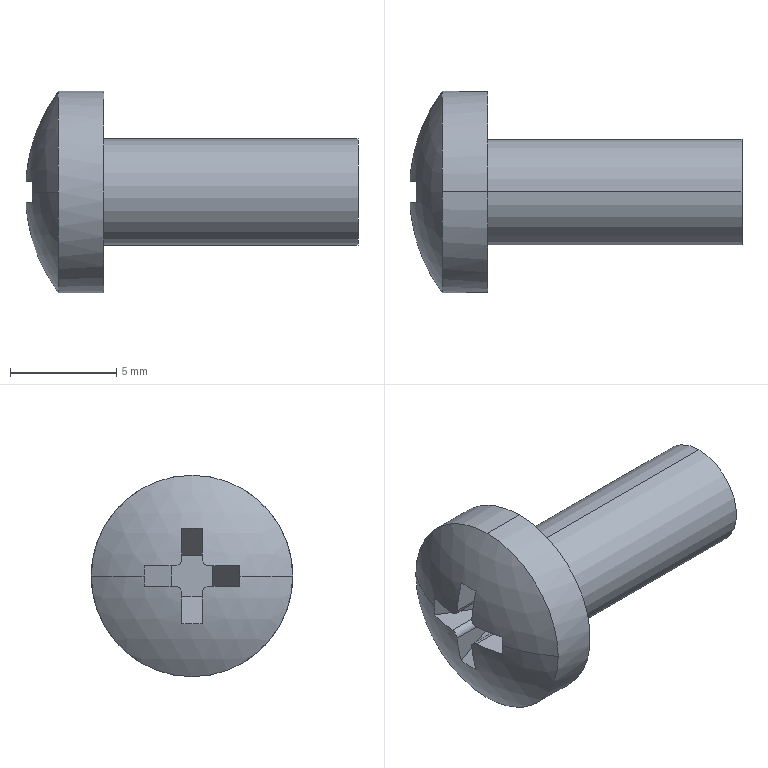Part | SolidWorks | features BaseBody 1 | 1 solid | 25 faces | box 15.658 x 9.5 x 9.5 mm | volume 430.614 mm3 | plane 15 | cylinder 8 | sphere 2 | commonest cylinder face diameters 0.6 x4 5 x2 9.5 x2
STEP:
#1=CARTESIAN_POINT('',(1.563,4.75,0.));
#2=VERTEX_POINT('',#1);
#3=CARTESIAN_POINT('',(1.563,0.,4.75));
#4=VERTEX_POINT('',#3);
#5=CARTESIAN_POINT('',(1.563,0.,0.));
#6=DIRECTION('',(1.,0.,0.));
#7=DIRECTION('',(0.,0.,-1.));
#8=AXIS2_PLACEMENT_3D('',#5,#6,#7);
#9=CIRCLE('',#8,4.75);
#10=EDGE_CURVE('',#2,#4,#9,.T.);
#11=ORIENTED_EDGE('',*,*,#10,.T.);
#12=CARTESIAN_POINT('',(3.7,0.,4.75));
#13=VERTEX_POINT('',#12);
#14=CARTESIAN_POINT('',(4.516,0.,4.75));
#15=DIRECTION('',(1.,0.,0.));
#16=VECTOR('',#15,1000.);
#17=LINE('',#14,#16);
#18=EDGE_CURVE('',#4,#13,#17,.T.);
#19=ORIENTED_EDGE('',*,*,#18,.T.);
#20=CARTESIAN_POINT('',(3.7,0.,-4.75));
#21=VERTEX_POINT('',#20);
#22=CARTESIAN_POINT('',(3.7,0.,0.));
#23=DIRECTION('',(1.,0.,0.));
#24=DIRECTION('',(0.,0.,-1.));
#25=AXIS2_PLACEMENT_3D('',#22,#23,#24);
#26=CIRCLE('',#25,4.75);
#27=EDGE_CURVE('',#21,#13,#26,.T.);
#28=ORIENTED_EDGE('',*,*,#27,.F.);
#29=CARTESIAN_POINT('',(1.563,0.,-4.75));
#30=VERTEX_POINT('',#29);
#31=CARTESIAN_POINT('',(4.516,0.,-4.75));
#32=DIRECTION('',(1.,0.,0.));
#33=VECTOR('',#32,1000.);
#34=LINE('',#31,#33);
#35=EDGE_CURVE('',#30,#21,#34,.T.);
#36=ORIENTED_EDGE('',*,*,#35,.F.);
#37=CARTESIAN_POINT('',(1.563,0.,0.));
#38=DIRECTION('',(1.,0.,0.));
#39=DIRECTION('',(0.,0.,-1.));
#40=AXIS2_PLACEMENT_3D('',#37,#38,#39);
#41=CIRCLE('',#40,4.75);
#42=EDGE_CURVE('',#30,#2,#41,.T.);
#43=ORIENTED_EDGE('',*,*,#42,.T.);
#44=EDGE_LOOP('',(#11,#19,#28,#36,#43));
#45=FACE_OUTER_BOUND('',#44,.T.);
#46=CARTESIAN_POINT('',(4.516,0.,0.));
#47=DIRECTION('',(1.,0.,0.));
#48=DIRECTION('',(0.,0.,-1.));
#49=AXIS2_PLACEMENT_3D('',#46,#47,#48);
#50=CYLINDRICAL_SURFACE('',#49,4.75);
#51=ADVANCED_FACE('',(#45),#50,.T.);
#52=CARTESIAN_POINT('',(3.7,0.,-2.5));
#53=VERTEX_POINT('',#52);
#54=CARTESIAN_POINT('',(3.7,0.,2.5));
#55=VERTEX_POINT('',#54);
#56=CARTESIAN_POINT('',(3.7,0.,0.));
#57=DIRECTION('',(1.,0.,0.));
#58=DIRECTION('',(0.,0.,-1.));
#59=AXIS2_PLACEMENT_3D('',#56,#57,#58);
#60=CIRCLE('',#59,2.5);
#61=EDGE_CURVE('',#53,#55,#60,.T.);
#62=ORIENTED_EDGE('',*,*,#61,.T.);
#63=CARTESIAN_POINT('',(15.7,0.,2.5));
#64=VERTEX_POINT('',#63);
#65=CARTESIAN_POINT('',(4.516,0.,2.5));
#66=DIRECTION('',(1.,0.,0.));
#67=VECTOR('',#66,1000.);
#68=LINE('',#65,#67);
#69=EDGE_CURVE('',#55,#64,#68,.T.);
#70=ORIENTED_EDGE('',*,*,#69,.T.);
#71=CARTESIAN_POINT('',(15.7,0.,-2.5));
#72=VERTEX_POINT('',#71);
#73=CARTESIAN_POINT('',(15.7,0.,0.));
#74=DIRECTION('',(1.,0.,0.));
#75=DIRECTION('',(0.,0.,-1.));
#76=AXIS2_PLACEMENT_3D('',#73,#74,#75);
#77=CIRCLE('',#76,2.5);
#78=EDGE_CURVE('',#72,#64,#77,.T.);
#79=ORIENTED_EDGE('',*,*,#78,.F.);
#80=CARTESIAN_POINT('',(4.516,0.,-2.5));
#81=DIRECTION('',(1.,0.,0.));
#82=VECTOR('',#81,1000.);
#83=LINE('',#80,#82);
#84=EDGE_CURVE('',#53,#72,#83,.T.);
#85=ORIENTED_EDGE('',*,*,#84,.F.);
#86=EDGE_LOOP('',(#62,#70,#79,#85));
#87=FACE_OUTER_BOUND('',#86,.T.);
#88=CARTESIAN_POINT('',(4.516,0.,0.));
#89=DIRECTION('',(1.,0.,0.));
#90=DIRECTION('',(0.,0.,-1.));
#91=AXIS2_PLACEMENT_3D('',#88,#89,#90);
#92=CYLINDRICAL_SURFACE('',#91,2.5);
#93=ADVANCED_FACE('',(#87),#92,.T.);
#94=CARTESIAN_POINT('',(1.563,-4.75,0.));
#95=VERTEX_POINT('',#94);
#96=CARTESIAN_POINT('',(1.563,0.,0.));
#97=DIRECTION('',(1.,0.,0.));
#98=DIRECTION('',(0.,0.,-1.));
#99=AXIS2_PLACEMENT_3D('',#96,#97,#98);
#100=CIRCLE('',#99,4.75);
#101=EDGE_CURVE('',#95,#30,#100,.T.);
#102=ORIENTED_EDGE('',*,*,#101,.F.);
#103=CARTESIAN_POINT('',(0.3263,-2.262,0.));
#104=VERTEX_POINT('',#103);
#105=CARTESIAN_POINT('',(8.,0.,0.));
#106=DIRECTION('',(0.,0.,-1.));
#107=DIRECTION('',(0.,1.,0.));
#108=AXIS2_PLACEMENT_3D('',#105,#106,#107);
#109=CIRCLE('',#108,8.);
#110=EDGE_CURVE('',#95,#104,#109,.T.);
#111=ORIENTED_EDGE('',*,*,#110,.T.);
#112=CARTESIAN_POINT('',(0.3397,-2.254,-0.49));
#113=VERTEX_POINT('',#112);
#114=CARTESIAN_POINT('',(7.061,1.627,0.));
#115=DIRECTION('',(0.5,-0.866,0.));
#116=DIRECTION('',(-0.866,-0.5,0.));
#117=AXIS2_PLACEMENT_3D('',#114,#115,#116);
#118=CIRCLE('',#117,7.776);
#119=EDGE_CURVE('',#104,#113,#118,.T.);
#120=ORIENTED_EDGE('',*,*,#119,.T.);
#121=CARTESIAN_POINT('',(0.0542,-0.79,-0.49));
#122=VERTEX_POINT('',#121);
#123=CARTESIAN_POINT('',(8.,0.,-0.49));
#124=DIRECTION('',(0.,0.,-1.));
#125=DIRECTION('',(1.,0.,0.));
#126=AXIS2_PLACEMENT_3D('',#123,#124,#125);
#127=CIRCLE('',#126,7.985);
#128=EDGE_CURVE('',#113,#122,#127,.T.);
#129=ORIENTED_EDGE('',*,*,#128,.T.);
#130=CARTESIAN_POINT('',(0.0542,-0.49,-0.79));
#131=VERTEX_POINT('',#130);
#132=CARTESIAN_POINT('',(0.0542,-0.79,-0.49));
#133=CARTESIAN_POINT('',(0.04634,-0.711,-0.49));
#134=CARTESIAN_POINT('',(0.04186,-0.6334,-0.5224));
#135=CARTESIAN_POINT('',(0.04185,-0.5225,-0.6332));
#136=CARTESIAN_POINT('',(0.04634,-0.49,-0.711));
#137=CARTESIAN_POINT('',(0.0542,-0.49,-0.79));
#138=B_SPLINE_CURVE_WITH_KNOTS('',3,(#132,#133,#134,#135,#136,#137),.UNSPECIFIED.,.F.,.F.,(4,2,4),(0.,0.0002348,0.0004695),.UNSPECIFIED.);
#139=EDGE_CURVE('',#122,#131,#138,.T.);
#140=ORIENTED_EDGE('',*,*,#139,.T.);
#141=CARTESIAN_POINT('',(0.3397,-0.49,-2.254));
#142=VERTEX_POINT('',#141);
#143=CARTESIAN_POINT('',(8.,-0.49,0.));
#144=DIRECTION('',(0.,-1.,0.));
#145=DIRECTION('',(0.,0.,1.));
#146=AXIS2_PLACEMENT_3D('',#143,#144,#145);
#147=CIRCLE('',#146,7.985);
#148=EDGE_CURVE('',#131,#142,#147,.T.);
#149=ORIENTED_EDGE('',*,*,#148,.T.);
#150=CARTESIAN_POINT('',(0.3397,0.49,-2.254));
#151=VERTEX_POINT('',#150);
#152=CARTESIAN_POINT('',(7.061,0.,1.627));
#153=DIRECTION('',(0.5,0.,-0.866));
#154=DIRECTION('',(0.866,0.,0.5));
#155=AXIS2_PLACEMENT_3D('',#152,#153,#154);
#156=CIRCLE('',#155,7.776);
#157=EDGE_CURVE('',#142,#151,#156,.T.);
#158=ORIENTED_EDGE('',*,*,#157,.T.);
#159=CARTESIAN_POINT('',(0.0542,0.49,-0.79));
#160=VERTEX_POINT('',#159);
#161=CARTESIAN_POINT('',(8.,0.49,0.));
#162=DIRECTION('',(0.,1.,0.));
#163=DIRECTION('',(0.,0.,-1.));
#164=AXIS2_PLACEMENT_3D('',#161,#162,#163);
#165=CIRCLE('',#164,7.985);
#166=EDGE_CURVE('',#151,#160,#165,.T.);
#167=ORIENTED_EDGE('',*,*,#166,.T.);
#168=CARTESIAN_POINT('',(0.0542,0.79,-0.49));
#169=VERTEX_POINT('',#168);
#170=CARTESIAN_POINT('',(0.0542,0.49,-0.79));
#171=CARTESIAN_POINT('',(0.04634,0.49,-0.711));
#172=CARTESIAN_POINT('',(0.04186,0.5224,-0.6334));
#173=CARTESIAN_POINT('',(0.04185,0.6332,-0.5225));
#174=CARTESIAN_POINT('',(0.04634,0.711,-0.49));
#175=CARTESIAN_POINT('',(0.0542,0.79,-0.49));
#176=B_SPLINE_CURVE_WITH_KNOTS('',3,(#170,#171,#172,#173,#174,#175),.UNSPECIFIED.,.F.,.F.,(4,2,4),(0.,0.0002348,0.0004695),.UNSPECIFIED.);
#177=EDGE_CURVE('',#160,#169,#176,.T.);
#178=ORIENTED_EDGE('',*,*,#177,.T.);
#179=CARTESIAN_POINT('',(0.3397,2.254,-0.49));
#180=VERTEX_POINT('',#179);
#181=CARTESIAN_POINT('',(8.,0.,-0.49));
#182=DIRECTION('',(0.,0.,-1.));
#183=DIRECTION('',(1.,0.,0.));
#184=AXIS2_PLACEMENT_3D('',#181,#182,#183);
#185=CIRCLE('',#184,7.985);
#186=EDGE_CURVE('',#169,#180,#185,.T.);
#187=ORIENTED_EDGE('',*,*,#186,.T.);
#188=CARTESIAN_POINT('',(0.3263,2.262,0.));
#189=VERTEX_POINT('',#188);
#190=CARTESIAN_POINT('',(7.061,-1.627,0.));
#191=DIRECTION('',(0.5,0.866,0.));
#192=DIRECTION('',(0.866,-0.5,0.));
#193=AXIS2_PLACEMENT_3D('',#190,#191,#192);
#194=CIRCLE('',#193,7.776);
#195=EDGE_CURVE('',#180,#189,#194,.T.);
#196=ORIENTED_EDGE('',*,*,#195,.T.);
#197=CARTESIAN_POINT('',(8.,0.,0.));
#198=DIRECTION('',(0.,0.,1.));
#199=DIRECTION('',(1.,0.,0.));
#200=AXIS2_PLACEMENT_3D('',#197,#198,#199);
#201=CIRCLE('',#200,8.);
#202=EDGE_CURVE('',#2,#189,#201,.T.);
#203=ORIENTED_EDGE('',*,*,#202,.F.);
#204=ORIENTED_EDGE('',*,*,#42,.F.);
#205=EDGE_LOOP('',(#102,#111,#120,#129,#140,#149,#158,#167,#178,#187,#196,#203,#204));
#206=FACE_OUTER_BOUND('',#205,.T.);
#207=CARTESIAN_POINT('',(8.,0.,0.));
#208=DIRECTION('',(0.,0.,-1.));
#209=DIRECTION('',(0.,1.,0.));
#210=AXIS2_PLACEMENT_3D('',#207,#208,#209);
#211=SPHERICAL_SURFACE('',#210,8.);
#212=ADVANCED_FACE('',(#206),#211,.T.);
#213=CARTESIAN_POINT('',(2.59,0.79,-0.49));
#214=VERTEX_POINT('',#213);
#215=CARTESIAN_POINT('',(2.59,0.49,-0.79));
#216=VERTEX_POINT('',#215);
#217=CARTESIAN_POINT('',(2.59,0.79,-0.79));
#218=DIRECTION('',(1.,0.,0.));
#219=DIRECTION('',(0.,0.,-1.));
#220=AXIS2_PLACEMENT_3D('',#217,#218,#219);
#221=CIRCLE('',#220,0.3);
#222=EDGE_CURVE('',#214,#216,#221,.T.);
#223=ORIENTED_EDGE('',*,*,#222,.F.);
#224=CARTESIAN_POINT('',(2.59,0.79,-0.49));
#225=DIRECTION('',(1.,0.,0.));
#226=VECTOR('',#225,1000.);
#227=LINE('',#224,#226);
#228=EDGE_CURVE('',#169,#214,#227,.T.);
#229=ORIENTED_EDGE('',*,*,#228,.F.);
#230=ORIENTED_EDGE('',*,*,#177,.F.);
#231=CARTESIAN_POINT('',(2.59,0.49,-0.79));
#232=DIRECTION('',(-1.,0.,0.));
#233=VECTOR('',#232,1000.);
#234=LINE('',#231,#233);
#235=EDGE_CURVE('',#216,#160,#234,.T.);
#236=ORIENTED_EDGE('',*,*,#235,.F.);
#237=EDGE_LOOP('',(#223,#229,#230,#236));
#238=FACE_OUTER_BOUND('',#237,.T.);
#239=CARTESIAN_POINT('',(2.59,0.79,-0.79));
#240=DIRECTION('',(-1.,0.,0.));
#241=DIRECTION('',(0.,0.,1.));
#242=AXIS2_PLACEMENT_3D('',#239,#240,#241);
#243=CYLINDRICAL_SURFACE('',#242,0.3);
#244=ADVANCED_FACE('',(#238),#243,.T.);
#245=CARTESIAN_POINT('',(2.59,0.49,0.79));
#246=VERTEX_POINT('',#245);
#247=CARTESIAN_POINT('',(2.59,0.79,0.49));
#248=VERTEX_POINT('',#247);
#249=CARTESIAN_POINT('',(2.59,0.79,0.79));
#250=DIRECTION('',(1.,0.,0.));
#251=DIRECTION('',(0.,0.,-1.));
#252=AXIS2_PLACEMENT_3D('',#249,#250,#251);
#253=CIRCLE('',#252,0.3);
#254=EDGE_CURVE('',#246,#248,#253,.T.);
#255=ORIENTED_EDGE('',*,*,#254,.F.);
#256=CARTESIAN_POINT('',(0.0542,0.49,0.79));
#257=VERTEX_POINT('',#256);
#258=CARTESIAN_POINT('',(2.59,0.49,0.79));
#259=DIRECTION('',(1.,0.,0.));
#260=VECTOR('',#259,1000.);
#261=LINE('',#258,#260);
#262=EDGE_CURVE('',#257,#246,#261,.T.);
#263=ORIENTED_EDGE('',*,*,#262,.F.);
#264=CARTESIAN_POINT('',(0.0542,0.79,0.49));
#265=VERTEX_POINT('',#264);
#266=CARTESIAN_POINT('',(0.0542,0.79,0.49));
#267=CARTESIAN_POINT('',(0.04634,0.711,0.49));
#268=CARTESIAN_POINT('',(0.04186,0.6334,0.5224));
#269=CARTESIAN_POINT('',(0.04185,0.5225,0.6332));
#270=CARTESIAN_POINT('',(0.04634,0.49,0.711));
#271=CARTESIAN_POINT('',(0.0542,0.49,0.79));
#272=B_SPLINE_CURVE_WITH_KNOTS('',3,(#266,#267,#268,#269,#270,#271),.UNSPECIFIED.,.F.,.F.,(4,2,4),(0.,0.0002348,0.0004695),.UNSPECIFIED.);
#273=EDGE_CURVE('',#265,#257,#272,.T.);
#274=ORIENTED_EDGE('',*,*,#273,.F.);
#275=CARTESIAN_POINT('',(2.59,0.79,0.49));
#276=DIRECTION('',(-1.,0.,0.));
#277=VECTOR('',#276,1000.);
#278=LINE('',#275,#277);
#279=EDGE_CURVE('',#248,#265,#278,.T.);
#280=ORIENTED_EDGE('',*,*,#279,.F.);
#281=EDGE_LOOP('',(#255,#263,#274,#280));
#282=FACE_OUTER_BOUND('',#281,.T.);
#283=CARTESIAN_POINT('',(2.59,0.79,0.79));
#284=DIRECTION('',(-1.,0.,0.));
#285=DIRECTION('',(0.,0.,1.));
#286=AXIS2_PLACEMENT_3D('',#283,#284,#285);
#287=CYLINDRICAL_SURFACE('',#286,0.3);
#288=ADVANCED_FACE('',(#282),#287,.T.);
#289=CARTESIAN_POINT('',(2.59,-0.49,-0.79));
#290=VERTEX_POINT('',#289);
#291=CARTESIAN_POINT('',(2.59,-0.79,-0.49));
#292=VERTEX_POINT('',#291);
#293=CARTESIAN_POINT('',(2.59,-0.79,-0.79));
#294=DIRECTION('',(1.,0.,0.));
#295=DIRECTION('',(0.,0.,-1.));
#296=AXIS2_PLACEMENT_3D('',#293,#294,#295);
#297=CIRCLE('',#296,0.3);
#298=EDGE_CURVE('',#290,#292,#297,.T.);
#299=ORIENTED_EDGE('',*,*,#298,.F.);
#300=CARTESIAN_POINT('',(2.59,-0.49,-0.79));
#301=DIRECTION('',(1.,0.,0.));
#302=VECTOR('',#301,1000.);
#303=LINE('',#300,#302);
#304=EDGE_CURVE('',#131,#290,#303,.T.);
#305=ORIENTED_EDGE('',*,*,#304,.F.);
#306=ORIENTED_EDGE('',*,*,#139,.F.);
#307=CARTESIAN_POINT('',(2.59,-0.79,-0.49));
#308=DIRECTION('',(-1.,0.,0.));
#309=VECTOR('',#308,1000.);
#310=LINE('',#307,#309);
#311=EDGE_CURVE('',#292,#122,#310,.T.);
#312=ORIENTED_EDGE('',*,*,#311,.F.);
#313=EDGE_LOOP('',(#299,#305,#306,#312));
#314=FACE_OUTER_BOUND('',#313,.T.);
#315=CARTESIAN_POINT('',(2.59,-0.79,-0.79));
#316=DIRECTION('',(-1.,0.,0.));
#317=DIRECTION('',(0.,0.,1.));
#318=AXIS2_PLACEMENT_3D('',#315,#316,#317);
#319=CYLINDRICAL_SURFACE('',#318,0.3);
#320=ADVANCED_FACE('',(#314),#319,.T.);
#321=CARTESIAN_POINT('',(2.59,-0.79,0.49));
#322=VERTEX_POINT('',#321);
#323=CARTESIAN_POINT('',(2.59,-0.49,0.79));
#324=VERTEX_POINT('',#323);
#325=CARTESIAN_POINT('',(2.59,-0.79,0.79));
#326=DIRECTION('',(1.,0.,0.));
#327=DIRECTION('',(0.,0.,-1.));
#328=AXIS2_PLACEMENT_3D('',#325,#326,#327);
#329=CIRCLE('',#328,0.3);
#330=EDGE_CURVE('',#322,#324,#329,.T.);
#331=ORIENTED_EDGE('',*,*,#330,.F.);
#332=CARTESIAN_POINT('',(0.0542,-0.79,0.49));
#333=VERTEX_POINT('',#332);
#334=CARTESIAN_POINT('',(2.59,-0.79,0.49));
#335=DIRECTION('',(1.,0.,0.));
#336=VECTOR('',#335,1000.);
#337=LINE('',#334,#336);
#338=EDGE_CURVE('',#333,#322,#337,.T.);
#339=ORIENTED_EDGE('',*,*,#338,.F.);
#340=CARTESIAN_POINT('',(0.0542,-0.49,0.79));
#341=VERTEX_POINT('',#340);
#342=CARTESIAN_POINT('',(0.0542,-0.49,0.79));
#343=CARTESIAN_POINT('',(0.04634,-0.49,0.711));
#344=CARTESIAN_POINT('',(0.04186,-0.5224,0.6334));
#345=CARTESIAN_POINT('',(0.04185,-0.6332,0.5225));
#346=CARTESIAN_POINT('',(0.04634,-0.711,0.49));
#347=CARTESIAN_POINT('',(0.0542,-0.79,0.49));
#348=B_SPLINE_CURVE_WITH_KNOTS('',3,(#342,#343,#344,#345,#346,#347),.UNSPECIFIED.,.F.,.F.,(4,2,4),(0.,0.0002348,0.0004695),.UNSPECIFIED.);
#349=EDGE_CURVE('',#341,#333,#348,.T.);
#350=ORIENTED_EDGE('',*,*,#349,.F.);
#351=CARTESIAN_POINT('',(2.59,-0.49,0.79));
#352=DIRECTION('',(-1.,0.,0.));
#353=VECTOR('',#352,1000.);
#354=LINE('',#351,#353);
#355=EDGE_CURVE('',#324,#341,#354,.T.);
#356=ORIENTED_EDGE('',*,*,#355,.F.);
#357=EDGE_LOOP('',(#331,#339,#350,#356));
#358=FACE_OUTER_BOUND('',#357,.T.);
#359=CARTESIAN_POINT('',(2.59,-0.79,0.79));
#360=DIRECTION('',(-1.,0.,0.));
#361=DIRECTION('',(0.,0.,1.));
#362=AXIS2_PLACEMENT_3D('',#359,#360,#361);
#363=CYLINDRICAL_SURFACE('',#362,0.3);
#364=ADVANCED_FACE('',(#358),#363,.T.);
#365=CARTESIAN_POINT('',(2.59,0.49,0.9547));
#366=VERTEX_POINT('',#365);
#367=CARTESIAN_POINT('',(2.59,0.49,0.49));
#368=DIRECTION('',(0.,0.,1.));
#369=VECTOR('',#368,1000.);
#370=LINE('',#367,#369);
#371=EDGE_CURVE('',#246,#366,#370,.T.);
#372=ORIENTED_EDGE('',*,*,#371,.F.);
#373=ORIENTED_EDGE('',*,*,#254,.T.);
#374=CARTESIAN_POINT('',(2.59,0.9547,0.49));
#375=VERTEX_POINT('',#374);
#376=CARTESIAN_POINT('',(2.59,0.49,0.49));
#377=DIRECTION('',(0.,-1.,0.));
#378=VECTOR('',#377,1000.);
#379=LINE('',#376,#378);
#380=EDGE_CURVE('',#375,#248,#379,.T.);
#381=ORIENTED_EDGE('',*,*,#380,.F.);
#382=CARTESIAN_POINT('',(2.59,0.9547,-0.49));
#383=VERTEX_POINT('',#382);
#384=CARTESIAN_POINT('',(2.59,0.9547,0.));
#385=DIRECTION('',(0.,0.,1.));
#386=VECTOR('',#385,1000.);
#387=LINE('',#384,#386);
#388=EDGE_CURVE('',#383,#375,#387,.T.);
#389=ORIENTED_EDGE('',*,*,#388,.F.);
#390=CARTESIAN_POINT('',(2.59,0.49,-0.49));
#391=DIRECTION('',(0.,1.,0.));
#392=VECTOR('',#391,1000.);
#393=LINE('',#390,#392);
#394=EDGE_CURVE('',#214,#383,#393,.T.);
#395=ORIENTED_EDGE('',*,*,#394,.F.);
#396=ORIENTED_EDGE('',*,*,#222,.T.);
#397=CARTESIAN_POINT('',(2.59,0.49,-0.9547));
#398=VERTEX_POINT('',#397);
#399=CARTESIAN_POINT('',(2.59,0.49,-0.49));
#400=DIRECTION('',(0.,0.,1.));
#401=VECTOR('',#400,1000.);
#402=LINE('',#399,#401);
#403=EDGE_CURVE('',#398,#216,#402,.T.);
#404=ORIENTED_EDGE('',*,*,#403,.F.);
#405=CARTESIAN_POINT('',(2.59,-0.49,-0.9547));
#406=VERTEX_POINT('',#405);
#407=CARTESIAN_POINT('',(2.59,0.,-0.9547));
#408=DIRECTION('',(0.,1.,0.));
#409=VECTOR('',#408,1000.);
#410=LINE('',#407,#409);
#411=EDGE_CURVE('',#406,#398,#410,.T.);
#412=ORIENTED_EDGE('',*,*,#411,.F.);
#413=CARTESIAN_POINT('',(2.59,-0.49,-0.49));
#414=DIRECTION('',(0.,0.,-1.));
#415=VECTOR('',#414,1000.);
#416=LINE('',#413,#415);
#417=EDGE_CURVE('',#290,#406,#416,.T.);
#418=ORIENTED_EDGE('',*,*,#417,.F.);
#419=ORIENTED_EDGE('',*,*,#298,.T.);
#420=CARTESIAN_POINT('',(2.59,-0.9547,-0.49));
#421=VERTEX_POINT('',#420);
#422=CARTESIAN_POINT('',(2.59,-0.49,-0.49));
#423=DIRECTION('',(0.,1.,0.));
#424=VECTOR('',#423,1000.);
#425=LINE('',#422,#424);
#426=EDGE_CURVE('',#421,#292,#425,.T.);
#427=ORIENTED_EDGE('',*,*,#426,.F.);
#428=CARTESIAN_POINT('',(2.59,-0.9547,0.49));
#429=VERTEX_POINT('',#428);
#430=CARTESIAN_POINT('',(2.59,-0.9547,0.));
#431=DIRECTION('',(0.,0.,-1.));
#432=VECTOR('',#431,1000.);
#433=LINE('',#430,#432);
#434=EDGE_CURVE('',#429,#421,#433,.T.);
#435=ORIENTED_EDGE('',*,*,#434,.F.);
#436=CARTESIAN_POINT('',(2.59,-0.49,0.49));
#437=DIRECTION('',(0.,-1.,0.));
#438=VECTOR('',#437,1000.);
#439=LINE('',#436,#438);
#440=EDGE_CURVE('',#322,#429,#439,.T.);
#441=ORIENTED_EDGE('',*,*,#440,.F.);
#442=ORIENTED_EDGE('',*,*,#330,.T.);
#443=CARTESIAN_POINT('',(2.59,-0.49,0.9547));
#444=VERTEX_POINT('',#443);
#445=CARTESIAN_POINT('',(2.59,-0.49,0.49));
#446=DIRECTION('',(0.,0.,-1.));
#447=VECTOR('',#446,1000.);
#448=LINE('',#445,#447);
#449=EDGE_CURVE('',#444,#324,#448,.T.);
#450=ORIENTED_EDGE('',*,*,#449,.F.);
#451=CARTESIAN_POINT('',(2.59,0.,0.9547));
#452=DIRECTION('',(0.,-1.,0.));
#453=VECTOR('',#452,1000.);
#454=LINE('',#451,#453);
#455=EDGE_CURVE('',#366,#444,#454,.T.);
#456=ORIENTED_EDGE('',*,*,#455,.F.);
#457=EDGE_LOOP('',(#372,#373,#381,#389,#395,#396,#404,#412,#418,#419,#427,#435,#441,#442,#450,#456));
#458=FACE_OUTER_BOUND('',#457,.T.);
#459=CARTESIAN_POINT('',(2.59,0.49,0.49));
#460=DIRECTION('',(1.,0.,0.));
#461=DIRECTION('',(0.,1.,0.));
#462=AXIS2_PLACEMENT_3D('',#459,#460,#461);
#463=PLANE('',#462);
#464=ADVANCED_FACE('',(#458),#463,.F.);
#465=ORIENTED_EDGE('',*,*,#380,.T.);
#466=ORIENTED_EDGE('',*,*,#279,.T.);
#467=CARTESIAN_POINT('',(0.3397,2.254,0.49));
#468=VERTEX_POINT('',#467);
#469=CARTESIAN_POINT('',(8.,0.,0.49));
#470=DIRECTION('',(0.,0.,1.));
#471=DIRECTION('',(0.,1.,0.));
#472=AXIS2_PLACEMENT_3D('',#469,#470,#471);
#473=CIRCLE('',#472,7.985);
#474=EDGE_CURVE('',#468,#265,#473,.T.);
#475=ORIENTED_EDGE('',*,*,#474,.F.);
#476=CARTESIAN_POINT('',(2.791,0.8385,0.49));
#477=DIRECTION('',(-0.866,0.5,0.));
#478=VECTOR('',#477,1000.);
#479=LINE('',#476,#478);
#480=EDGE_CURVE('',#375,#468,#479,.T.);
#481=ORIENTED_EDGE('',*,*,#480,.F.);
#482=EDGE_LOOP('',(#465,#466,#475,#481));
#483=FACE_OUTER_BOUND('',#482,.T.);
#484=CARTESIAN_POINT('',(2.59,0.49,0.49));
#485=DIRECTION('',(0.,0.,-1.));
#486=DIRECTION('',(-1.,0.,0.));
#487=AXIS2_PLACEMENT_3D('',#484,#485,#486);
#488=PLANE('',#487);
#489=ADVANCED_FACE('',(#483),#488,.T.);
#490=CARTESIAN_POINT('',(0.,2.45,-0.49));
#491=DIRECTION('',(-0.866,0.5,0.));
#492=VECTOR('',#491,1000.);
#493=LINE('',#490,#492);
#494=EDGE_CURVE('',#383,#180,#493,.T.);
#495=ORIENTED_EDGE('',*,*,#494,.F.);
#496=ORIENTED_EDGE('',*,*,#388,.T.);
#497=ORIENTED_EDGE('',*,*,#480,.T.);
#498=CARTESIAN_POINT('',(7.061,-1.627,0.));
#499=DIRECTION('',(0.5,0.866,0.));
#500=DIRECTION('',(0.866,-0.5,0.));
#501=AXIS2_PLACEMENT_3D('',#498,#499,#500);
#502=CIRCLE('',#501,7.776);
#503=EDGE_CURVE('',#189,#468,#502,.T.);
#504=ORIENTED_EDGE('',*,*,#503,.F.);
#505=ORIENTED_EDGE('',*,*,#195,.F.);
#506=EDGE_LOOP('',(#495,#496,#497,#504,#505));
#507=FACE_OUTER_BOUND('',#506,.T.);
#508=CARTESIAN_POINT('',(0.,2.45,0.));
#509=DIRECTION('',(-0.5,-0.866,0.));
#510=DIRECTION('',(-0.866,0.5,0.));
#511=AXIS2_PLACEMENT_3D('',#508,#509,#510);
#512=PLANE('',#511);
#513=ADVANCED_FACE('',(#507),#512,.T.);
#514=ORIENTED_EDGE('',*,*,#186,.F.);
#515=ORIENTED_EDGE('',*,*,#228,.T.);
#516=ORIENTED_EDGE('',*,*,#394,.T.);
#517=ORIENTED_EDGE('',*,*,#494,.T.);
#518=EDGE_LOOP('',(#514,#515,#516,#517));
#519=FACE_OUTER_BOUND('',#518,.T.);
#520=CARTESIAN_POINT('',(2.59,0.49,-0.49));
#521=DIRECTION('',(0.,0.,1.));
#522=DIRECTION('',(1.,0.,0.));
#523=AXIS2_PLACEMENT_3D('',#520,#521,#522);
#524=PLANE('',#523);
#525=ADVANCED_FACE('',(#519),#524,.T.);
#526=ORIENTED_EDGE('',*,*,#403,.T.);
#527=ORIENTED_EDGE('',*,*,#235,.T.);
#528=ORIENTED_EDGE('',*,*,#166,.F.);
#529=CARTESIAN_POINT('',(2.791,0.49,-0.8385));
#530=DIRECTION('',(-0.866,0.,-0.5));
#531=VECTOR('',#530,1000.);
#532=LINE('',#529,#531);
#533=EDGE_CURVE('',#398,#151,#532,.T.);
#534=ORIENTED_EDGE('',*,*,#533,.F.);
#535=EDGE_LOOP('',(#526,#527,#528,#534));
#536=FACE_OUTER_BOUND('',#535,.T.);
#537=CARTESIAN_POINT('',(2.59,0.49,-0.49));
#538=DIRECTION('',(0.,-1.,0.));
#539=DIRECTION('',(0.,0.,-1.));
#540=AXIS2_PLACEMENT_3D('',#537,#538,#539);
#541=PLANE('',#540);
#542=ADVANCED_FACE('',(#536),#541,.T.);
#543=CARTESIAN_POINT('',(0.,-0.49,-2.45));
#544=DIRECTION('',(-0.866,0.,-0.5));
#545=VECTOR('',#544,1000.);
#546=LINE('',#543,#545);
#547=EDGE_CURVE('',#406,#142,#546,.T.);
#548=ORIENTED_EDGE('',*,*,#547,.F.);
#549=ORIENTED_EDGE('',*,*,#411,.T.);
#550=ORIENTED_EDGE('',*,*,#533,.T.);
#551=ORIENTED_EDGE('',*,*,#157,.F.);
#552=EDGE_LOOP('',(#548,#549,#550,#551));
#553=FACE_OUTER_BOUND('',#552,.T.);
#554=CARTESIAN_POINT('',(0.,0.,-2.45));
#555=DIRECTION('',(-0.5,0.,0.866));
#556=DIRECTION('',(0.,1.,0.));
#557=AXIS2_PLACEMENT_3D('',#554,#555,#556);
#558=PLANE('',#557);
#559=ADVANCED_FACE('',(#553),#558,.T.);
#560=ORIENTED_EDGE('',*,*,#148,.F.);
#561=ORIENTED_EDGE('',*,*,#304,.T.);
#562=ORIENTED_EDGE('',*,*,#417,.T.);
#563=ORIENTED_EDGE('',*,*,#547,.T.);
#564=EDGE_LOOP('',(#560,#561,#562,#563));
#565=FACE_OUTER_BOUND('',#564,.T.);
#566=CARTESIAN_POINT('',(2.59,-0.49,-0.49));
#567=DIRECTION('',(0.,1.,0.));
#568=DIRECTION('',(1.,0.,0.));
#569=AXIS2_PLACEMENT_3D('',#566,#567,#568);
#570=PLANE('',#569);
#571=ADVANCED_FACE('',(#565),#570,.T.);
#572=ORIENTED_EDGE('',*,*,#426,.T.);
#573=ORIENTED_EDGE('',*,*,#311,.T.);
#574=ORIENTED_EDGE('',*,*,#128,.F.);
#575=CARTESIAN_POINT('',(2.791,-0.8385,-0.49));
#576=DIRECTION('',(-0.866,-0.5,0.));
#577=VECTOR('',#576,1000.);
#578=LINE('',#575,#577);
#579=EDGE_CURVE('',#421,#113,#578,.T.);
#580=ORIENTED_EDGE('',*,*,#579,.F.);
#581=EDGE_LOOP('',(#572,#573,#574,#580));
#582=FACE_OUTER_BOUND('',#581,.T.);
#583=CARTESIAN_POINT('',(2.59,-0.49,-0.49));
#584=DIRECTION('',(0.,0.,1.));
#585=DIRECTION('',(1.,0.,0.));
#586=AXIS2_PLACEMENT_3D('',#583,#584,#585);
#587=PLANE('',#586);
#588=ADVANCED_FACE('',(#582),#587,.T.);
#589=CARTESIAN_POINT('',(0.3397,-2.254,0.49));
#590=VERTEX_POINT('',#589);
#591=CARTESIAN_POINT('',(0.,-2.45,0.49));
#592=DIRECTION('',(-0.866,-0.5,0.));
#593=VECTOR('',#592,1000.);
#594=LINE('',#591,#593);
#595=EDGE_CURVE('',#429,#590,#594,.T.);
#596=ORIENTED_EDGE('',*,*,#595,.F.);
#597=ORIENTED_EDGE('',*,*,#434,.T.);
#598=ORIENTED_EDGE('',*,*,#579,.T.);
#599=ORIENTED_EDGE('',*,*,#119,.F.);
#600=CARTESIAN_POINT('',(7.061,1.627,0.));
#601=DIRECTION('',(0.5,-0.866,0.));
#602=DIRECTION('',(-0.866,-0.5,0.));
#603=AXIS2_PLACEMENT_3D('',#600,#601,#602);
#604=CIRCLE('',#603,7.776);
#605=EDGE_CURVE('',#590,#104,#604,.T.);
#606=ORIENTED_EDGE('',*,*,#605,.F.);
#607=EDGE_LOOP('',(#596,#597,#598,#599,#606));
#608=FACE_OUTER_BOUND('',#607,.T.);
#609=CARTESIAN_POINT('',(0.,-2.45,0.));
#610=DIRECTION('',(-0.5,0.866,0.));
#611=DIRECTION('',(0.,0.,1.));
#612=AXIS2_PLACEMENT_3D('',#609,#610,#611);
#613=PLANE('',#612);
#614=ADVANCED_FACE('',(#608),#613,.T.);
#615=CARTESIAN_POINT('',(8.,0.,0.49));
#616=DIRECTION('',(0.,0.,1.));
#617=DIRECTION('',(0.,1.,0.));
#618=AXIS2_PLACEMENT_3D('',#615,#616,#617);
#619=CIRCLE('',#618,7.985);
#620=EDGE_CURVE('',#333,#590,#619,.T.);
#621=ORIENTED_EDGE('',*,*,#620,.F.);
#622=ORIENTED_EDGE('',*,*,#338,.T.);
#623=ORIENTED_EDGE('',*,*,#440,.T.);
#624=ORIENTED_EDGE('',*,*,#595,.T.);
#625=EDGE_LOOP('',(#621,#622,#623,#624));
#626=FACE_OUTER_BOUND('',#625,.T.);
#627=CARTESIAN_POINT('',(2.59,-0.49,0.49));
#628=DIRECTION('',(0.,0.,-1.));
#629=DIRECTION('',(-1.,0.,0.));
#630=AXIS2_PLACEMENT_3D('',#627,#628,#629);
#631=PLANE('',#630);
#632=ADVANCED_FACE('',(#626),#631,.T.);
#633=ORIENTED_EDGE('',*,*,#449,.T.);
#634=ORIENTED_EDGE('',*,*,#355,.T.);
#635=CARTESIAN_POINT('',(0.3397,-0.49,2.254));
#636=VERTEX_POINT('',#635);
#637=CARTESIAN_POINT('',(8.,-0.49,0.));
#638=DIRECTION('',(0.,-1.,0.));
#639=DIRECTION('',(0.,0.,1.));
#640=AXIS2_PLACEMENT_3D('',#637,#638,#639);
#641=CIRCLE('',#640,7.985);
#642=EDGE_CURVE('',#636,#341,#641,.T.);
#643=ORIENTED_EDGE('',*,*,#642,.F.);
#644=CARTESIAN_POINT('',(2.791,-0.49,0.8385));
#645=DIRECTION('',(-0.866,0.,0.5));
#646=VECTOR('',#645,1000.);
#647=LINE('',#644,#646);
#648=EDGE_CURVE('',#444,#636,#647,.T.);
#649=ORIENTED_EDGE('',*,*,#648,.F.);
#650=EDGE_LOOP('',(#633,#634,#643,#649));
#651=FACE_OUTER_BOUND('',#650,.T.);
#652=CARTESIAN_POINT('',(2.59,-0.49,0.49));
#653=DIRECTION('',(0.,1.,0.));
#654=DIRECTION('',(0.,0.,-1.));
#655=AXIS2_PLACEMENT_3D('',#652,#653,#654);
#656=PLANE('',#655);
#657=ADVANCED_FACE('',(#651),#656,.T.);
#658=CARTESIAN_POINT('',(0.3397,0.49,2.254));
#659=VERTEX_POINT('',#658);
#660=CARTESIAN_POINT('',(0.,0.49,2.45));
#661=DIRECTION('',(-0.866,0.,0.5));
#662=VECTOR('',#661,1000.);
#663=LINE('',#660,#662);
#664=EDGE_CURVE('',#366,#659,#663,.T.);
#665=ORIENTED_EDGE('',*,*,#664,.F.);
#666=ORIENTED_EDGE('',*,*,#455,.T.);
#667=ORIENTED_EDGE('',*,*,#648,.T.);
#668=CARTESIAN_POINT('',(7.061,0.,-1.627));
#669=DIRECTION('',(0.5,0.,0.866));
#670=DIRECTION('',(-0.866,0.,0.5));
#671=AXIS2_PLACEMENT_3D('',#668,#669,#670);
#672=CIRCLE('',#671,7.776);
#673=EDGE_CURVE('',#659,#636,#672,.T.);
#674=ORIENTED_EDGE('',*,*,#673,.F.);
#675=EDGE_LOOP('',(#665,#666,#667,#674));
#676=FACE_OUTER_BOUND('',#675,.T.);
#677=CARTESIAN_POINT('',(0.,0.,2.45));
#678=DIRECTION('',(-0.5,0.,-0.866));
#679=DIRECTION('',(-0.866,0.,0.5));
#680=AXIS2_PLACEMENT_3D('',#677,#678,#679);
#681=PLANE('',#680);
#682=ADVANCED_FACE('',(#676),#681,.T.);
#683=CARTESIAN_POINT('',(8.,0.49,0.));
#684=DIRECTION('',(0.,1.,0.));
#685=DIRECTION('',(0.,0.,-1.));
#686=AXIS2_PLACEMENT_3D('',#683,#684,#685);
#687=CIRCLE('',#686,7.985);
#688=EDGE_CURVE('',#257,#659,#687,.T.);
#689=ORIENTED_EDGE('',*,*,#688,.F.);
#690=ORIENTED_EDGE('',*,*,#262,.T.);
#691=ORIENTED_EDGE('',*,*,#371,.T.);
#692=ORIENTED_EDGE('',*,*,#664,.T.);
#693=EDGE_LOOP('',(#689,#690,#691,#692));
#694=FACE_OUTER_BOUND('',#693,.T.);
#695=CARTESIAN_POINT('',(2.59,0.49,0.49));
#696=DIRECTION('',(0.,-1.,0.));
#697=DIRECTION('',(0.,0.,-1.));
#698=AXIS2_PLACEMENT_3D('',#695,#696,#697);
#699=PLANE('',#698);
#700=ADVANCED_FACE('',(#694),#699,.T.);
#701=ORIENTED_EDGE('',*,*,#61,.F.);
#702=CARTESIAN_POINT('',(3.7,0.,0.));
#703=DIRECTION('',(1.,0.,0.));
#704=DIRECTION('',(0.,0.,-1.));
#705=AXIS2_PLACEMENT_3D('',#702,#703,#704);
#706=CIRCLE('',#705,2.5);
#707=EDGE_CURVE('',#55,#53,#706,.T.);
#708=ORIENTED_EDGE('',*,*,#707,.F.);
#709=EDGE_LOOP('',(#701,#708));
#710=FACE_BOUND('',#709,.T.);
#711=ORIENTED_EDGE('',*,*,#27,.T.);
#712=CARTESIAN_POINT('',(3.7,0.,0.));
#713=DIRECTION('',(1.,0.,0.));
#714=DIRECTION('',(0.,0.,-1.));
#715=AXIS2_PLACEMENT_3D('',#712,#713,#714);
#716=CIRCLE('',#715,4.75);
#717=EDGE_CURVE('',#13,#21,#716,.T.);
#718=ORIENTED_EDGE('',*,*,#717,.T.);
#719=EDGE_LOOP('',(#711,#718));
#720=FACE_OUTER_BOUND('',#719,.T.);
#721=CARTESIAN_POINT('',(3.7,2.85,0.));
#722=DIRECTION('',(1.,0.,0.));
#723=DIRECTION('',(0.,1.,0.));
#724=AXIS2_PLACEMENT_3D('',#721,#722,#723);
#725=PLANE('',#724);
#726=ADVANCED_FACE('',(#710,#720),#725,.T.);
#727=ORIENTED_EDGE('',*,*,#78,.T.);
#728=CARTESIAN_POINT('',(15.7,0.,0.));
#729=DIRECTION('',(1.,0.,0.));
#730=DIRECTION('',(0.,0.,-1.));
#731=AXIS2_PLACEMENT_3D('',#728,#729,#730);
#732=CIRCLE('',#731,2.5);
#733=EDGE_CURVE('',#64,#72,#732,.T.);
#734=ORIENTED_EDGE('',*,*,#733,.T.);
#735=EDGE_LOOP('',(#727,#734));
#736=FACE_OUTER_BOUND('',#735,.T.);
#737=CARTESIAN_POINT('',(15.7,2.5,0.));
#738=DIRECTION('',(1.,0.,0.));
#739=DIRECTION('',(0.,1.,0.));
#740=AXIS2_PLACEMENT_3D('',#737,#738,#739);
#741=PLANE('',#740);
#742=ADVANCED_FACE('',(#736),#741,.T.);
#743=ORIENTED_EDGE('',*,*,#110,.F.);
#744=CARTESIAN_POINT('',(1.563,0.,0.));
#745=DIRECTION('',(1.,0.,0.));
#746=DIRECTION('',(0.,0.,-1.));
#747=AXIS2_PLACEMENT_3D('',#744,#745,#746);
#748=CIRCLE('',#747,4.75);
#749=EDGE_CURVE('',#4,#95,#748,.T.);
#750=ORIENTED_EDGE('',*,*,#749,.F.);
#751=ORIENTED_EDGE('',*,*,#10,.F.);
#752=ORIENTED_EDGE('',*,*,#202,.T.);
#753=ORIENTED_EDGE('',*,*,#503,.T.);
#754=ORIENTED_EDGE('',*,*,#474,.T.);
#755=ORIENTED_EDGE('',*,*,#273,.T.);
#756=ORIENTED_EDGE('',*,*,#688,.T.);
#757=ORIENTED_EDGE('',*,*,#673,.T.);
#758=ORIENTED_EDGE('',*,*,#642,.T.);
#759=ORIENTED_EDGE('',*,*,#349,.T.);
#760=ORIENTED_EDGE('',*,*,#620,.T.);
#761=ORIENTED_EDGE('',*,*,#605,.T.);
#762=EDGE_LOOP('',(#743,#750,#751,#752,#753,#754,#755,#756,#757,#758,#759,#760,#761));
#763=FACE_OUTER_BOUND('',#762,.T.);
#764=CARTESIAN_POINT('',(8.,0.,0.));
#765=DIRECTION('',(0.,0.,-1.));
#766=DIRECTION('',(0.,1.,0.));
#767=AXIS2_PLACEMENT_3D('',#764,#765,#766);
#768=SPHERICAL_SURFACE('',#767,8.);
#769=ADVANCED_FACE('',(#763),#768,.T.);
#770=ORIENTED_EDGE('',*,*,#69,.F.);
#771=ORIENTED_EDGE('',*,*,#707,.T.);
#772=ORIENTED_EDGE('',*,*,#84,.T.);
#773=ORIENTED_EDGE('',*,*,#733,.F.);
#774=EDGE_LOOP('',(#770,#771,#772,#773));
#775=FACE_OUTER_BOUND('',#774,.T.);
#776=CARTESIAN_POINT('',(4.516,0.,0.));
#777=DIRECTION('',(1.,0.,0.));
#778=DIRECTION('',(0.,0.,-1.));
#779=AXIS2_PLACEMENT_3D('',#776,#777,#778);
#780=CYLINDRICAL_SURFACE('',#779,2.5);
#781=ADVANCED_FACE('',(#775),#780,.T.);
#782=ORIENTED_EDGE('',*,*,#18,.F.);
#783=ORIENTED_EDGE('',*,*,#749,.T.);
#784=ORIENTED_EDGE('',*,*,#101,.T.);
#785=ORIENTED_EDGE('',*,*,#35,.T.);
#786=ORIENTED_EDGE('',*,*,#717,.F.);
#787=EDGE_LOOP('',(#782,#783,#784,#785,#786));
#788=FACE_OUTER_BOUND('',#787,.T.);
#789=CARTESIAN_POINT('',(4.516,0.,0.));
#790=DIRECTION('',(1.,0.,0.));
#791=DIRECTION('',(0.,0.,-1.));
#792=AXIS2_PLACEMENT_3D('',#789,#790,#791);
#793=CYLINDRICAL_SURFACE('',#792,4.75);
#794=ADVANCED_FACE('',(#788),#793,.T.);
#795=CLOSED_SHELL('',(#51,#93,#212,#244,#288,#320,#364,#464,#489,#513,#525,#542,#559,#571,#588,#614,#632,#657,#682,#700,#726,#742,#769,#781,#794));
#796=MANIFOLD_SOLID_BREP('',#795);
#797=CARTESIAN_POINT('',(0.,0.,0.));
#798=DIRECTION('',(0.,0.,1.));
#799=DIRECTION('',(1.,0.,0.));
#800=AXIS2_PLACEMENT_3D('',#797,#798,#799);
#801=(LENGTH_UNIT()NAMED_UNIT(*)SI_UNIT(.MILLI.,.METRE.));
#802=UNCERTAINTY_MEASURE_WITH_UNIT(LENGTH_MEASURE(0.00001),#801,'','');
#803=(NAMED_UNIT(*)PLANE_ANGLE_UNIT()SI_UNIT($,.RADIAN.));
#804=(NAMED_UNIT(*)SI_UNIT($,.STERADIAN.)SOLID_ANGLE_UNIT());
#805=(GEOMETRIC_REPRESENTATION_CONTEXT(3)GLOBAL_UNCERTAINTY_ASSIGNED_CONTEXT((#802))GLOBAL_UNIT_ASSIGNED_CONTEXT((#801,#803,#804))REPRESENTATION_CONTEXT('',''));
#806=ADVANCED_BREP_SHAPE_REPRESENTATION('',(#796,#800),#805);